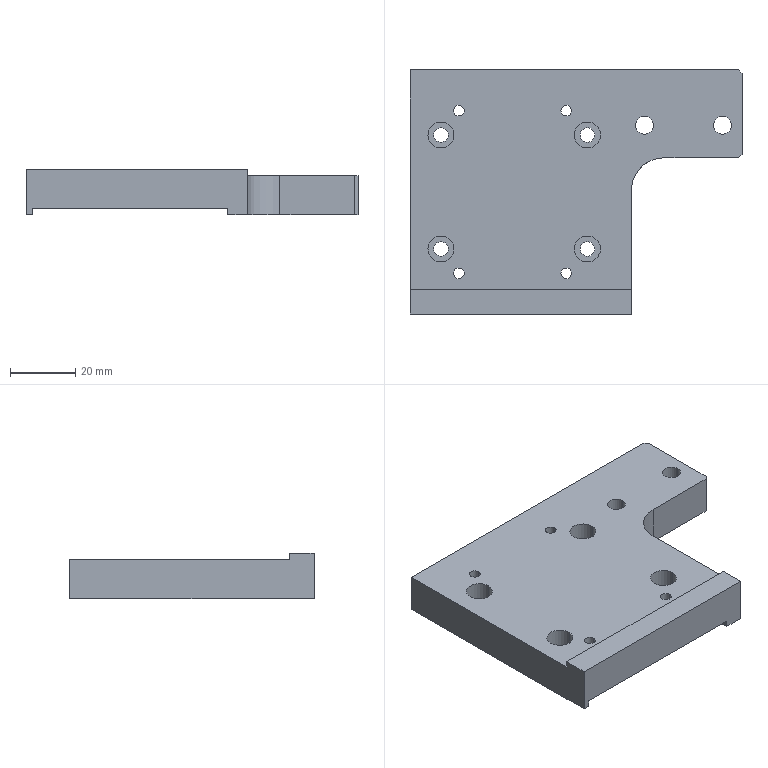Part | STEP file | 2036 Guide rail mounting plate | 1 solid | 55 faces | box 102 x 75 x 14 mm | volume 61484 mm3 | cylinder 33 | plane 22 | commonest cylinder face diameters 3.3 x8 4.5 x8 8 x8 5.5 x4 10 x4 20 x1